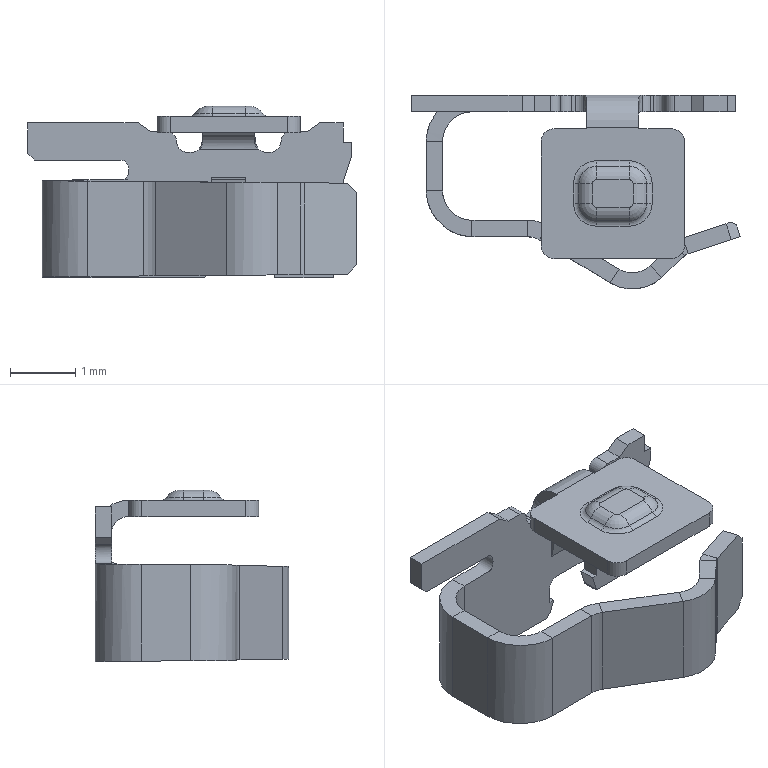Part | NX | 1 solid | 141 faces | box 5.018 x 2.959 x 2.622 mm | volume 5.784 mm3 | plane 89 | cylinder 38 | torus 12 | spline 2 | commonest cylinder face diameters 0.3 x6 0.2 x5 0.5 x5 0.7 x5 0.35 x4 0.4 x4